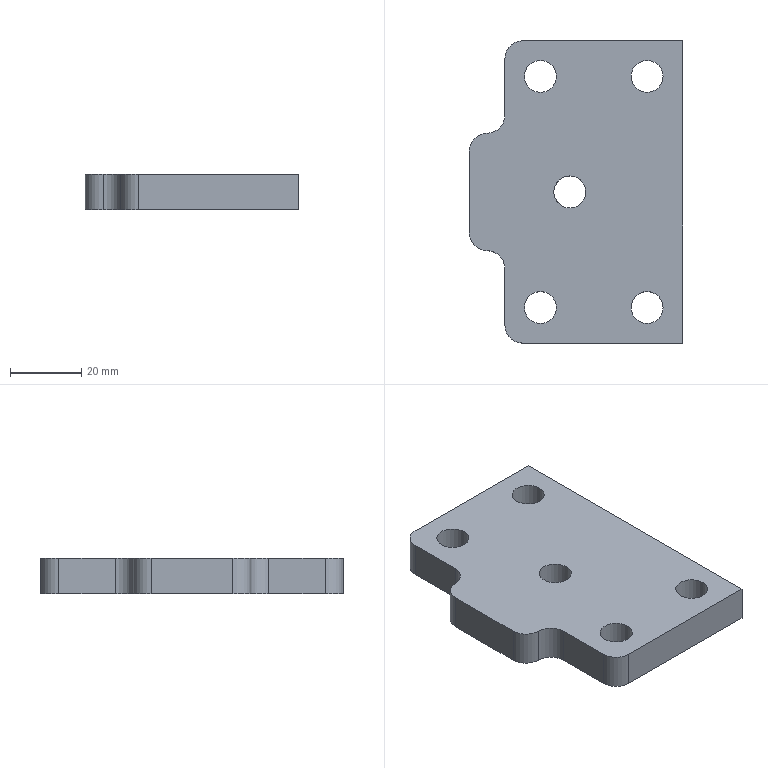Part | STEP file | PN_0048_id1026_x_t | 1 solid | 19 faces | box 60 x 85 x 10 mm | volume 42512 mm3 | cylinder 11 | plane 8 | commonest cylinder face diameters 10 x6 9 x5
STEP:
#1=CARTESIAN_POINT('',(294.75,11.5,105.));
#2=VERTEX_POINT('',#1);
#3=CARTESIAN_POINT('',(294.75,-11.5,105.));
#4=VERTEX_POINT('',#3);
#5=CARTESIAN_POINT('',(294.75,3.,105.));
#6=DIRECTION('',(0.,-1.,0.));
#7=VECTOR('',#6,1.);
#8=LINE('',#5,#7);
#9=EDGE_CURVE('',#2,#4,#8,.T.);
#10=ORIENTED_EDGE('',*,*,#9,.F.);
#11=CARTESIAN_POINT('',(294.75,11.5,95.));
#12=VERTEX_POINT('',#11);
#13=CARTESIAN_POINT('',(294.75,11.5,11.));
#14=DIRECTION('',(0.,0.,-1.));
#15=VECTOR('',#14,1.);
#16=LINE('',#13,#15);
#17=EDGE_CURVE('',#2,#12,#16,.T.);
#18=ORIENTED_EDGE('',*,*,#17,.T.);
#19=CARTESIAN_POINT('',(294.75,-11.5,95.));
#20=VERTEX_POINT('',#19);
#21=CARTESIAN_POINT('',(294.75,-13.,95.));
#22=DIRECTION('',(0.,-1.,0.));
#23=VECTOR('',#22,1.);
#24=LINE('',#21,#23);
#25=EDGE_CURVE('',#12,#20,#24,.T.);
#26=ORIENTED_EDGE('',*,*,#25,.T.);
#27=CARTESIAN_POINT('',(294.75,-11.5,105.));
#28=DIRECTION('',(0.,0.,1.));
#29=VECTOR('',#28,1.);
#30=LINE('',#27,#29);
#31=EDGE_CURVE('',#20,#4,#30,.T.);
#32=ORIENTED_EDGE('',*,*,#31,.T.);
#33=EDGE_LOOP('',(#10,#18,#26,#32));
#34=FACE_OUTER_BOUND('',#33,.T.);
#35=CARTESIAN_POINT('',(294.75,-13.,11.));
#36=DIRECTION('',(-1.,0.,0.));
#37=DIRECTION('',(0.,1.,0.));
#38=AXIS2_PLACEMENT_3D('',#35,#36,#37);
#39=PLANE('',#38);
#40=ADVANCED_FACE('',(#34),#39,.T.);
#41=CARTESIAN_POINT('',(354.75,-42.5,105.));
#42=VERTEX_POINT('',#41);
#43=CARTESIAN_POINT('',(309.75,-42.5,105.));
#44=VERTEX_POINT('',#43);
#45=CARTESIAN_POINT('',(546.19,-42.5,105.));
#46=DIRECTION('',(-1.,0.,0.));
#47=VECTOR('',#46,1.);
#48=LINE('',#45,#47);
#49=EDGE_CURVE('',#42,#44,#48,.T.);
#50=ORIENTED_EDGE('',*,*,#49,.T.);
#51=CARTESIAN_POINT('',(309.75,-42.5,95.));
#52=VERTEX_POINT('',#51);
#53=CARTESIAN_POINT('',(309.75,-42.5,95.));
#54=DIRECTION('',(0.,0.,-1.));
#55=VECTOR('',#54,1.);
#56=LINE('',#53,#55);
#57=EDGE_CURVE('',#44,#52,#56,.T.);
#58=ORIENTED_EDGE('',*,*,#57,.T.);
#59=CARTESIAN_POINT('',(354.75,-42.5,95.));
#60=VERTEX_POINT('',#59);
#61=CARTESIAN_POINT('',(265.5,-42.5,95.));
#62=DIRECTION('',(-1.,0.,0.));
#63=VECTOR('',#62,1.);
#64=LINE('',#61,#63);
#65=EDGE_CURVE('',#60,#52,#64,.T.);
#66=ORIENTED_EDGE('',*,*,#65,.F.);
#67=CARTESIAN_POINT('',(354.75,-42.5,11.));
#68=DIRECTION('',(0.,0.,1.));
#69=VECTOR('',#68,1.);
#70=LINE('',#67,#69);
#71=EDGE_CURVE('',#60,#42,#70,.T.);
#72=ORIENTED_EDGE('',*,*,#71,.T.);
#73=EDGE_LOOP('',(#50,#58,#66,#72));
#74=FACE_OUTER_BOUND('',#73,.T.);
#75=CARTESIAN_POINT('',(546.19,-42.5,11.));
#76=DIRECTION('',(0.,-1.,0.));
#77=DIRECTION('',(-1.,0.,0.));
#78=AXIS2_PLACEMENT_3D('',#75,#76,#77);
#79=PLANE('',#78);
#80=ADVANCED_FACE('',(#74),#79,.T.);
#81=CARTESIAN_POINT('',(354.75,42.5,95.));
#82=VERTEX_POINT('',#81);
#83=CARTESIAN_POINT('',(309.75,42.5,95.));
#84=VERTEX_POINT('',#83);
#85=CARTESIAN_POINT('',(265.5,42.5,95.));
#86=DIRECTION('',(-1.,0.,0.));
#87=VECTOR('',#86,1.);
#88=LINE('',#85,#87);
#89=EDGE_CURVE('',#82,#84,#88,.T.);
#90=ORIENTED_EDGE('',*,*,#89,.T.);
#91=CARTESIAN_POINT('',(309.75,42.5,105.));
#92=VERTEX_POINT('',#91);
#93=CARTESIAN_POINT('',(309.75,42.5,105.));
#94=DIRECTION('',(0.,0.,1.));
#95=VECTOR('',#94,1.);
#96=LINE('',#93,#95);
#97=EDGE_CURVE('',#84,#92,#96,.T.);
#98=ORIENTED_EDGE('',*,*,#97,.T.);
#99=CARTESIAN_POINT('',(354.75,42.5,105.));
#100=VERTEX_POINT('',#99);
#101=CARTESIAN_POINT('',(266.,42.5,105.));
#102=DIRECTION('',(-1.,0.,0.));
#103=VECTOR('',#102,1.);
#104=LINE('',#101,#103);
#105=EDGE_CURVE('',#100,#92,#104,.T.);
#106=ORIENTED_EDGE('',*,*,#105,.F.);
#107=CARTESIAN_POINT('',(354.75,42.5,11.));
#108=DIRECTION('',(0.,0.,1.));
#109=VECTOR('',#108,1.);
#110=LINE('',#107,#109);
#111=EDGE_CURVE('',#82,#100,#110,.T.);
#112=ORIENTED_EDGE('',*,*,#111,.F.);
#113=EDGE_LOOP('',(#90,#98,#106,#112));
#114=FACE_OUTER_BOUND('',#113,.T.);
#115=CARTESIAN_POINT('',(266.,42.5,11.));
#116=DIRECTION('',(0.,1.,0.));
#117=DIRECTION('',(1.,0.,0.));
#118=AXIS2_PLACEMENT_3D('',#115,#116,#117);
#119=PLANE('',#118);
#120=ADVANCED_FACE('',(#114),#119,.T.);
#121=CARTESIAN_POINT('',(323.,4.5,105.));
#122=VERTEX_POINT('',#121);
#123=CARTESIAN_POINT('',(323.,0.,105.));
#124=DIRECTION('',(0.,0.,-1.));
#125=DIRECTION('',(0.,1.,0.));
#126=AXIS2_PLACEMENT_3D('',#123,#124,#125);
#127=CIRCLE('',#126,4.5);
#128=EDGE_CURVE('',#122,#122,#127,.T.);
#129=ORIENTED_EDGE('',*,*,#128,.T.);
#130=EDGE_LOOP('',(#129));
#131=FACE_BOUND('',#130,.T.);
#132=CARTESIAN_POINT('',(319.25,-32.5,105.));
#133=VERTEX_POINT('',#132);
#134=CARTESIAN_POINT('',(314.75,-32.5,105.));
#135=DIRECTION('',(0.,0.,-1.));
#136=DIRECTION('',(1.,0.,0.));
#137=AXIS2_PLACEMENT_3D('',#134,#135,#136);
#138=CIRCLE('',#137,4.5);
#139=EDGE_CURVE('',#133,#133,#138,.T.);
#140=ORIENTED_EDGE('',*,*,#139,.T.);
#141=EDGE_LOOP('',(#140));
#142=FACE_BOUND('',#141,.T.);
#143=CARTESIAN_POINT('',(340.25,-32.5,105.));
#144=VERTEX_POINT('',#143);
#145=CARTESIAN_POINT('',(344.75,-32.5,105.));
#146=DIRECTION('',(0.,0.,1.));
#147=DIRECTION('',(-1.,0.,0.));
#148=AXIS2_PLACEMENT_3D('',#145,#146,#147);
#149=CIRCLE('',#148,4.5);
#150=EDGE_CURVE('',#144,#144,#149,.T.);
#151=ORIENTED_EDGE('',*,*,#150,.F.);
#152=EDGE_LOOP('',(#151));
#153=FACE_BOUND('',#152,.T.);
#154=CARTESIAN_POINT('',(319.25,32.5,105.));
#155=VERTEX_POINT('',#154);
#156=CARTESIAN_POINT('',(314.75,32.5,105.));
#157=DIRECTION('',(0.,0.,1.));
#158=DIRECTION('',(1.,0.,0.));
#159=AXIS2_PLACEMENT_3D('',#156,#157,#158);
#160=CIRCLE('',#159,4.5);
#161=EDGE_CURVE('',#155,#155,#160,.T.);
#162=ORIENTED_EDGE('',*,*,#161,.F.);
#163=EDGE_LOOP('',(#162));
#164=FACE_BOUND('',#163,.T.);
#165=CARTESIAN_POINT('',(340.25,32.5,105.));
#166=VERTEX_POINT('',#165);
#167=CARTESIAN_POINT('',(344.75,32.5,105.));
#168=DIRECTION('',(0.,0.,-1.));
#169=DIRECTION('',(-1.,0.,0.));
#170=AXIS2_PLACEMENT_3D('',#167,#168,#169);
#171=CIRCLE('',#170,4.5);
#172=EDGE_CURVE('',#166,#166,#171,.T.);
#173=ORIENTED_EDGE('',*,*,#172,.T.);
#174=EDGE_LOOP('',(#173));
#175=FACE_BOUND('',#174,.T.);
#176=ORIENTED_EDGE('',*,*,#105,.T.);
#177=CARTESIAN_POINT('',(304.75,37.5,105.));
#178=VERTEX_POINT('',#177);
#179=CARTESIAN_POINT('',(309.75,37.5,105.));
#180=DIRECTION('',(0.,0.,1.));
#181=DIRECTION('',(1.,0.,0.));
#182=AXIS2_PLACEMENT_3D('',#179,#180,#181);
#183=CIRCLE('',#182,5.);
#184=EDGE_CURVE('',#92,#178,#183,.T.);
#185=ORIENTED_EDGE('',*,*,#184,.T.);
#186=CARTESIAN_POINT('',(304.75,21.5,105.));
#187=VERTEX_POINT('',#186);
#188=CARTESIAN_POINT('',(304.75,3.,105.));
#189=DIRECTION('',(0.,-1.,0.));
#190=VECTOR('',#189,1.);
#191=LINE('',#188,#190);
#192=EDGE_CURVE('',#178,#187,#191,.T.);
#193=ORIENTED_EDGE('',*,*,#192,.T.);
#194=CARTESIAN_POINT('',(299.75,16.5,105.));
#195=VERTEX_POINT('',#194);
#196=CARTESIAN_POINT('',(299.75,21.5,105.));
#197=DIRECTION('',(0.,0.,-1.));
#198=DIRECTION('',(1.,0.,0.));
#199=AXIS2_PLACEMENT_3D('',#196,#197,#198);
#200=CIRCLE('',#199,5.);
#201=EDGE_CURVE('',#187,#195,#200,.T.);
#202=ORIENTED_EDGE('',*,*,#201,.T.);
#203=CARTESIAN_POINT('',(299.75,11.5,105.));
#204=DIRECTION('',(0.,0.,1.));
#205=DIRECTION('',(1.,0.,0.));
#206=AXIS2_PLACEMENT_3D('',#203,#204,#205);
#207=CIRCLE('',#206,5.);
#208=EDGE_CURVE('',#195,#2,#207,.T.);
#209=ORIENTED_EDGE('',*,*,#208,.T.);
#210=ORIENTED_EDGE('',*,*,#9,.T.);
#211=CARTESIAN_POINT('',(299.75,-16.5,105.));
#212=VERTEX_POINT('',#211);
#213=CARTESIAN_POINT('',(299.75,-11.5,105.));
#214=DIRECTION('',(0.,0.,1.));
#215=DIRECTION('',(1.,0.,0.));
#216=AXIS2_PLACEMENT_3D('',#213,#214,#215);
#217=CIRCLE('',#216,5.);
#218=EDGE_CURVE('',#4,#212,#217,.T.);
#219=ORIENTED_EDGE('',*,*,#218,.T.);
#220=CARTESIAN_POINT('',(304.75,-21.5,105.));
#221=VERTEX_POINT('',#220);
#222=CARTESIAN_POINT('',(299.75,-21.5,105.));
#223=DIRECTION('',(0.,0.,1.));
#224=DIRECTION('',(1.,0.,0.));
#225=AXIS2_PLACEMENT_3D('',#222,#223,#224);
#226=CIRCLE('',#225,5.);
#227=EDGE_CURVE('',#221,#212,#226,.T.);
#228=ORIENTED_EDGE('',*,*,#227,.F.);
#229=CARTESIAN_POINT('',(304.75,-37.5,105.));
#230=VERTEX_POINT('',#229);
#231=CARTESIAN_POINT('',(304.75,3.,105.));
#232=DIRECTION('',(0.,1.,0.));
#233=VECTOR('',#232,1.);
#234=LINE('',#231,#233);
#235=EDGE_CURVE('',#230,#221,#234,.T.);
#236=ORIENTED_EDGE('',*,*,#235,.F.);
#237=CARTESIAN_POINT('',(309.75,-37.5,105.));
#238=DIRECTION('',(0.,0.,1.));
#239=DIRECTION('',(1.,0.,0.));
#240=AXIS2_PLACEMENT_3D('',#237,#238,#239);
#241=CIRCLE('',#240,5.);
#242=EDGE_CURVE('',#230,#44,#241,.T.);
#243=ORIENTED_EDGE('',*,*,#242,.T.);
#244=ORIENTED_EDGE('',*,*,#49,.F.);
#245=CARTESIAN_POINT('',(354.75,52.192,105.));
#246=DIRECTION('',(0.,-1.,0.));
#247=VECTOR('',#246,1.);
#248=LINE('',#245,#247);
#249=EDGE_CURVE('',#100,#42,#248,.T.);
#250=ORIENTED_EDGE('',*,*,#249,.F.);
#251=EDGE_LOOP('',(#176,#185,#193,#202,#209,#210,#219,#228,#236,#243,#244,#250));
#252=FACE_BOUND('',#251,.T.);
#253=CARTESIAN_POINT('',(-321.,3.,105.));
#254=DIRECTION('',(0.,0.,1.));
#255=DIRECTION('',(1.,0.,0.));
#256=AXIS2_PLACEMENT_3D('',#253,#254,#255);
#257=PLANE('',#256);
#258=ADVANCED_FACE('',(#131,#142,#153,#164,#175,#252),#257,.T.);
#259=CARTESIAN_POINT('',(318.5,0.,95.));
#260=VERTEX_POINT('',#259);
#261=CARTESIAN_POINT('',(323.,0.,95.));
#262=DIRECTION('',(0.,0.,-1.));
#263=DIRECTION('',(-1.,0.,0.));
#264=AXIS2_PLACEMENT_3D('',#261,#262,#263);
#265=CIRCLE('',#264,4.5);
#266=EDGE_CURVE('',#260,#260,#265,.T.);
#267=ORIENTED_EDGE('',*,*,#266,.F.);
#268=EDGE_LOOP('',(#267));
#269=FACE_BOUND('',#268,.T.);
#270=CARTESIAN_POINT('',(310.25,-32.5,95.));
#271=VERTEX_POINT('',#270);
#272=CARTESIAN_POINT('',(314.75,-32.5,95.));
#273=DIRECTION('',(0.,0.,-1.));
#274=DIRECTION('',(-1.,0.,0.));
#275=AXIS2_PLACEMENT_3D('',#272,#273,#274);
#276=CIRCLE('',#275,4.5);
#277=EDGE_CURVE('',#271,#271,#276,.T.);
#278=ORIENTED_EDGE('',*,*,#277,.F.);
#279=EDGE_LOOP('',(#278));
#280=FACE_BOUND('',#279,.T.);
#281=CARTESIAN_POINT('',(340.25,-32.5,95.));
#282=VERTEX_POINT('',#281);
#283=CARTESIAN_POINT('',(344.75,-32.5,95.));
#284=DIRECTION('',(0.,0.,-1.));
#285=DIRECTION('',(-1.,0.,0.));
#286=AXIS2_PLACEMENT_3D('',#283,#284,#285);
#287=CIRCLE('',#286,4.5);
#288=EDGE_CURVE('',#282,#282,#287,.T.);
#289=ORIENTED_EDGE('',*,*,#288,.F.);
#290=EDGE_LOOP('',(#289));
#291=FACE_BOUND('',#290,.T.);
#292=CARTESIAN_POINT('',(310.25,32.5,95.));
#293=VERTEX_POINT('',#292);
#294=CARTESIAN_POINT('',(314.75,32.5,95.));
#295=DIRECTION('',(0.,0.,-1.));
#296=DIRECTION('',(-1.,0.,0.));
#297=AXIS2_PLACEMENT_3D('',#294,#295,#296);
#298=CIRCLE('',#297,4.5);
#299=EDGE_CURVE('',#293,#293,#298,.T.);
#300=ORIENTED_EDGE('',*,*,#299,.F.);
#301=EDGE_LOOP('',(#300));
#302=FACE_BOUND('',#301,.T.);
#303=CARTESIAN_POINT('',(340.25,32.5,95.));
#304=VERTEX_POINT('',#303);
#305=CARTESIAN_POINT('',(344.75,32.5,95.));
#306=DIRECTION('',(0.,0.,-1.));
#307=DIRECTION('',(-1.,0.,0.));
#308=AXIS2_PLACEMENT_3D('',#305,#306,#307);
#309=CIRCLE('',#308,4.5);
#310=EDGE_CURVE('',#304,#304,#309,.T.);
#311=ORIENTED_EDGE('',*,*,#310,.F.);
#312=EDGE_LOOP('',(#311));
#313=FACE_BOUND('',#312,.T.);
#314=CARTESIAN_POINT('',(304.75,21.5,95.));
#315=VERTEX_POINT('',#314);
#316=CARTESIAN_POINT('',(304.75,37.5,95.));
#317=VERTEX_POINT('',#316);
#318=CARTESIAN_POINT('',(304.75,3.,95.));
#319=DIRECTION('',(0.,1.,0.));
#320=VECTOR('',#319,1.);
#321=LINE('',#318,#320);
#322=EDGE_CURVE('',#315,#317,#321,.T.);
#323=ORIENTED_EDGE('',*,*,#322,.T.);
#324=CARTESIAN_POINT('',(309.75,37.5,95.));
#325=DIRECTION('',(0.,0.,-1.));
#326=DIRECTION('',(-1.,0.,0.));
#327=AXIS2_PLACEMENT_3D('',#324,#325,#326);
#328=CIRCLE('',#327,5.);
#329=EDGE_CURVE('',#317,#84,#328,.T.);
#330=ORIENTED_EDGE('',*,*,#329,.T.);
#331=ORIENTED_EDGE('',*,*,#89,.F.);
#332=CARTESIAN_POINT('',(354.75,3.,95.));
#333=DIRECTION('',(0.,-1.,0.));
#334=VECTOR('',#333,1.);
#335=LINE('',#332,#334);
#336=EDGE_CURVE('',#82,#60,#335,.T.);
#337=ORIENTED_EDGE('',*,*,#336,.T.);
#338=ORIENTED_EDGE('',*,*,#65,.T.);
#339=CARTESIAN_POINT('',(304.75,-37.5,95.));
#340=VERTEX_POINT('',#339);
#341=CARTESIAN_POINT('',(309.75,-37.5,95.));
#342=DIRECTION('',(0.,0.,-1.));
#343=DIRECTION('',(-1.,0.,0.));
#344=AXIS2_PLACEMENT_3D('',#341,#342,#343);
#345=CIRCLE('',#344,5.);
#346=EDGE_CURVE('',#52,#340,#345,.T.);
#347=ORIENTED_EDGE('',*,*,#346,.T.);
#348=CARTESIAN_POINT('',(304.75,-21.5,95.));
#349=VERTEX_POINT('',#348);
#350=CARTESIAN_POINT('',(304.75,3.,95.));
#351=DIRECTION('',(0.,-1.,0.));
#352=VECTOR('',#351,1.);
#353=LINE('',#350,#352);
#354=EDGE_CURVE('',#349,#340,#353,.T.);
#355=ORIENTED_EDGE('',*,*,#354,.F.);
#356=CARTESIAN_POINT('',(299.75,-16.5,95.));
#357=VERTEX_POINT('',#356);
#358=CARTESIAN_POINT('',(299.75,-21.5,95.));
#359=DIRECTION('',(0.,0.,-1.));
#360=DIRECTION('',(-1.,0.,0.));
#361=AXIS2_PLACEMENT_3D('',#358,#359,#360);
#362=CIRCLE('',#361,5.);
#363=EDGE_CURVE('',#357,#349,#362,.T.);
#364=ORIENTED_EDGE('',*,*,#363,.F.);
#365=CARTESIAN_POINT('',(299.75,-11.5,95.));
#366=DIRECTION('',(0.,0.,-1.));
#367=DIRECTION('',(-1.,0.,0.));
#368=AXIS2_PLACEMENT_3D('',#365,#366,#367);
#369=CIRCLE('',#368,5.);
#370=EDGE_CURVE('',#357,#20,#369,.T.);
#371=ORIENTED_EDGE('',*,*,#370,.T.);
#372=ORIENTED_EDGE('',*,*,#25,.F.);
#373=CARTESIAN_POINT('',(299.75,16.5,95.));
#374=VERTEX_POINT('',#373);
#375=CARTESIAN_POINT('',(299.75,11.5,95.));
#376=DIRECTION('',(0.,0.,-1.));
#377=DIRECTION('',(-1.,0.,0.));
#378=AXIS2_PLACEMENT_3D('',#375,#376,#377);
#379=CIRCLE('',#378,5.);
#380=EDGE_CURVE('',#12,#374,#379,.T.);
#381=ORIENTED_EDGE('',*,*,#380,.T.);
#382=CARTESIAN_POINT('',(299.75,21.5,95.));
#383=DIRECTION('',(0.,0.,1.));
#384=DIRECTION('',(-1.,0.,0.));
#385=AXIS2_PLACEMENT_3D('',#382,#383,#384);
#386=CIRCLE('',#385,5.);
#387=EDGE_CURVE('',#374,#315,#386,.T.);
#388=ORIENTED_EDGE('',*,*,#387,.T.);
#389=EDGE_LOOP('',(#323,#330,#331,#337,#338,#347,#355,#364,#371,#372,#381,#388));
#390=FACE_BOUND('',#389,.T.);
#391=CARTESIAN_POINT('',(265.5,3.,95.));
#392=DIRECTION('',(0.,0.,-1.));
#393=DIRECTION('',(-1.,0.,0.));
#394=AXIS2_PLACEMENT_3D('',#391,#392,#393);
#395=PLANE('',#394);
#396=ADVANCED_FACE('',(#269,#280,#291,#302,#313,#390),#395,.T.);
#397=ORIENTED_EDGE('',*,*,#111,.T.);
#398=ORIENTED_EDGE('',*,*,#249,.T.);
#399=ORIENTED_EDGE('',*,*,#71,.F.);
#400=ORIENTED_EDGE('',*,*,#336,.F.);
#401=EDGE_LOOP('',(#397,#398,#399,#400));
#402=FACE_OUTER_BOUND('',#401,.T.);
#403=CARTESIAN_POINT('',(354.75,52.192,11.));
#404=DIRECTION('',(-1.,0.,0.));
#405=DIRECTION('',(0.,1.,0.));
#406=AXIS2_PLACEMENT_3D('',#403,#404,#405);
#407=PLANE('',#406);
#408=ADVANCED_FACE('',(#402),#407,.F.);
#409=ORIENTED_EDGE('',*,*,#201,.F.);
#410=CARTESIAN_POINT('',(304.75,21.5,44.));
#411=DIRECTION('',(0.,0.,1.));
#412=VECTOR('',#411,1.);
#413=LINE('',#410,#412);
#414=EDGE_CURVE('',#315,#187,#413,.T.);
#415=ORIENTED_EDGE('',*,*,#414,.F.);
#416=ORIENTED_EDGE('',*,*,#387,.F.);
#417=CARTESIAN_POINT('',(299.75,16.5,44.));
#418=DIRECTION('',(0.,0.,1.));
#419=VECTOR('',#418,1.);
#420=LINE('',#417,#419);
#421=EDGE_CURVE('',#374,#195,#420,.T.);
#422=ORIENTED_EDGE('',*,*,#421,.T.);
#423=EDGE_LOOP('',(#409,#415,#416,#422));
#424=FACE_OUTER_BOUND('',#423,.T.);
#425=CARTESIAN_POINT('',(299.75,21.5,44.));
#426=DIRECTION('',(0.,0.,1.));
#427=DIRECTION('',(1.,0.,0.));
#428=AXIS2_PLACEMENT_3D('',#425,#426,#427);
#429=CYLINDRICAL_SURFACE('',#428,5.);
#430=ADVANCED_FACE('',(#424),#429,.F.);
#431=ORIENTED_EDGE('',*,*,#192,.F.);
#432=CARTESIAN_POINT('',(304.75,37.5,44.));
#433=DIRECTION('',(0.,0.,-1.));
#434=VECTOR('',#433,1.);
#435=LINE('',#432,#434);
#436=EDGE_CURVE('',#178,#317,#435,.T.);
#437=ORIENTED_EDGE('',*,*,#436,.T.);
#438=ORIENTED_EDGE('',*,*,#322,.F.);
#439=ORIENTED_EDGE('',*,*,#414,.T.);
#440=EDGE_LOOP('',(#431,#437,#438,#439));
#441=FACE_OUTER_BOUND('',#440,.T.);
#442=CARTESIAN_POINT('',(304.75,52.5,44.));
#443=DIRECTION('',(-1.,0.,0.));
#444=DIRECTION('',(0.,0.,1.));
#445=AXIS2_PLACEMENT_3D('',#442,#443,#444);
#446=PLANE('',#445);
#447=ADVANCED_FACE('',(#441),#446,.T.);
#448=ORIENTED_EDGE('',*,*,#227,.T.);
#449=CARTESIAN_POINT('',(299.75,-16.5,118.));
#450=DIRECTION('',(0.,0.,1.));
#451=VECTOR('',#450,1.);
#452=LINE('',#449,#451);
#453=EDGE_CURVE('',#357,#212,#452,.T.);
#454=ORIENTED_EDGE('',*,*,#453,.F.);
#455=ORIENTED_EDGE('',*,*,#363,.T.);
#456=CARTESIAN_POINT('',(304.75,-21.5,118.));
#457=DIRECTION('',(0.,0.,1.));
#458=VECTOR('',#457,1.);
#459=LINE('',#456,#458);
#460=EDGE_CURVE('',#349,#221,#459,.T.);
#461=ORIENTED_EDGE('',*,*,#460,.T.);
#462=EDGE_LOOP('',(#448,#454,#455,#461));
#463=FACE_OUTER_BOUND('',#462,.T.);
#464=CARTESIAN_POINT('',(299.75,-21.5,118.));
#465=DIRECTION('',(0.,0.,-1.));
#466=DIRECTION('',(-1.,0.,0.));
#467=AXIS2_PLACEMENT_3D('',#464,#465,#466);
#468=CYLINDRICAL_SURFACE('',#467,5.);
#469=ADVANCED_FACE('',(#463),#468,.F.);
#470=ORIENTED_EDGE('',*,*,#354,.T.);
#471=CARTESIAN_POINT('',(304.75,-37.5,11.));
#472=DIRECTION('',(0.,0.,1.));
#473=VECTOR('',#472,1.);
#474=LINE('',#471,#473);
#475=EDGE_CURVE('',#340,#230,#474,.T.);
#476=ORIENTED_EDGE('',*,*,#475,.T.);
#477=ORIENTED_EDGE('',*,*,#235,.T.);
#478=ORIENTED_EDGE('',*,*,#460,.F.);
#479=EDGE_LOOP('',(#470,#476,#477,#478));
#480=FACE_OUTER_BOUND('',#479,.T.);
#481=CARTESIAN_POINT('',(304.75,-52.5,118.));
#482=DIRECTION('',(1.,0.,0.));
#483=DIRECTION('',(0.,0.,-1.));
#484=AXIS2_PLACEMENT_3D('',#481,#482,#483);
#485=PLANE('',#484);
#486=ADVANCED_FACE('',(#480),#485,.F.);
#487=ORIENTED_EDGE('',*,*,#184,.F.);
#488=ORIENTED_EDGE('',*,*,#97,.F.);
#489=ORIENTED_EDGE('',*,*,#329,.F.);
#490=ORIENTED_EDGE('',*,*,#436,.F.);
#491=EDGE_LOOP('',(#487,#488,#489,#490));
#492=FACE_OUTER_BOUND('',#491,.T.);
#493=CARTESIAN_POINT('',(309.75,37.5,44.));
#494=DIRECTION('',(0.,0.,-1.));
#495=DIRECTION('',(-1.,0.,0.));
#496=AXIS2_PLACEMENT_3D('',#493,#494,#495);
#497=CYLINDRICAL_SURFACE('',#496,5.);
#498=ADVANCED_FACE('',(#492),#497,.T.);
#499=ORIENTED_EDGE('',*,*,#380,.F.);
#500=ORIENTED_EDGE('',*,*,#17,.F.);
#501=ORIENTED_EDGE('',*,*,#208,.F.);
#502=ORIENTED_EDGE('',*,*,#421,.F.);
#503=EDGE_LOOP('',(#499,#500,#501,#502));
#504=FACE_OUTER_BOUND('',#503,.T.);
#505=CARTESIAN_POINT('',(299.75,11.5,44.));
#506=DIRECTION('',(0.,0.,1.));
#507=DIRECTION('',(1.,0.,0.));
#508=AXIS2_PLACEMENT_3D('',#505,#506,#507);
#509=CYLINDRICAL_SURFACE('',#508,5.);
#510=ADVANCED_FACE('',(#504),#509,.T.);
#511=ORIENTED_EDGE('',*,*,#242,.F.);
#512=ORIENTED_EDGE('',*,*,#475,.F.);
#513=ORIENTED_EDGE('',*,*,#346,.F.);
#514=ORIENTED_EDGE('',*,*,#57,.F.);
#515=EDGE_LOOP('',(#511,#512,#513,#514));
#516=FACE_OUTER_BOUND('',#515,.T.);
#517=CARTESIAN_POINT('',(309.75,-37.5,11.));
#518=DIRECTION('',(0.,0.,1.));
#519=DIRECTION('',(1.,0.,0.));
#520=AXIS2_PLACEMENT_3D('',#517,#518,#519);
#521=CYLINDRICAL_SURFACE('',#520,5.);
#522=ADVANCED_FACE('',(#516),#521,.T.);
#523=ORIENTED_EDGE('',*,*,#370,.F.);
#524=ORIENTED_EDGE('',*,*,#453,.T.);
#525=ORIENTED_EDGE('',*,*,#218,.F.);
#526=ORIENTED_EDGE('',*,*,#31,.F.);
#527=EDGE_LOOP('',(#523,#524,#525,#526));
#528=FACE_OUTER_BOUND('',#527,.T.);
#529=CARTESIAN_POINT('',(299.75,-11.5,11.));
#530=DIRECTION('',(0.,0.,-1.));
#531=DIRECTION('',(-1.,0.,0.));
#532=AXIS2_PLACEMENT_3D('',#529,#530,#531);
#533=CYLINDRICAL_SURFACE('',#532,5.);
#534=ADVANCED_FACE('',(#528),#533,.T.);
#535=ORIENTED_EDGE('',*,*,#310,.T.);
#536=EDGE_LOOP('',(#535));
#537=FACE_BOUND('',#536,.T.);
#538=ORIENTED_EDGE('',*,*,#172,.F.);
#539=EDGE_LOOP('',(#538));
#540=FACE_BOUND('',#539,.T.);
#541=CARTESIAN_POINT('',(344.75,32.5,105.));
#542=DIRECTION('',(0.,0.,-1.));
#543=DIRECTION('',(-1.,0.,0.));
#544=AXIS2_PLACEMENT_3D('',#541,#542,#543);
#545=CYLINDRICAL_SURFACE('',#544,4.5);
#546=ADVANCED_FACE('',(#537,#540),#545,.F.);
#547=ORIENTED_EDGE('',*,*,#299,.T.);
#548=EDGE_LOOP('',(#547));
#549=FACE_BOUND('',#548,.T.);
#550=ORIENTED_EDGE('',*,*,#161,.T.);
#551=EDGE_LOOP('',(#550));
#552=FACE_BOUND('',#551,.T.);
#553=CARTESIAN_POINT('',(314.75,32.5,105.));
#554=DIRECTION('',(0.,0.,-1.));
#555=DIRECTION('',(1.,0.,0.));
#556=AXIS2_PLACEMENT_3D('',#553,#554,#555);
#557=CYLINDRICAL_SURFACE('',#556,4.5);
#558=ADVANCED_FACE('',(#549,#552),#557,.F.);
#559=ORIENTED_EDGE('',*,*,#288,.T.);
#560=EDGE_LOOP('',(#559));
#561=FACE_BOUND('',#560,.T.);
#562=ORIENTED_EDGE('',*,*,#150,.T.);
#563=EDGE_LOOP('',(#562));
#564=FACE_BOUND('',#563,.T.);
#565=CARTESIAN_POINT('',(344.75,-32.5,105.));
#566=DIRECTION('',(0.,0.,-1.));
#567=DIRECTION('',(-1.,0.,0.));
#568=AXIS2_PLACEMENT_3D('',#565,#566,#567);
#569=CYLINDRICAL_SURFACE('',#568,4.5);
#570=ADVANCED_FACE('',(#561,#564),#569,.F.);
#571=ORIENTED_EDGE('',*,*,#277,.T.);
#572=EDGE_LOOP('',(#571));
#573=FACE_BOUND('',#572,.T.);
#574=ORIENTED_EDGE('',*,*,#139,.F.);
#575=EDGE_LOOP('',(#574));
#576=FACE_BOUND('',#575,.T.);
#577=CARTESIAN_POINT('',(314.75,-32.5,105.));
#578=DIRECTION('',(0.,0.,-1.));
#579=DIRECTION('',(1.,0.,0.));
#580=AXIS2_PLACEMENT_3D('',#577,#578,#579);
#581=CYLINDRICAL_SURFACE('',#580,4.5);
#582=ADVANCED_FACE('',(#573,#576),#581,.F.);
#583=ORIENTED_EDGE('',*,*,#266,.T.);
#584=EDGE_LOOP('',(#583));
#585=FACE_BOUND('',#584,.T.);
#586=ORIENTED_EDGE('',*,*,#128,.F.);
#587=EDGE_LOOP('',(#586));
#588=FACE_BOUND('',#587,.T.);
#589=CARTESIAN_POINT('',(323.,0.,105.));
#590=DIRECTION('',(0.,0.,-1.));
#591=DIRECTION('',(0.,1.,0.));
#592=AXIS2_PLACEMENT_3D('',#589,#590,#591);
#593=CYLINDRICAL_SURFACE('',#592,4.5);
#594=ADVANCED_FACE('',(#585,#588),#593,.F.);
#595=CLOSED_SHELL('',(#40,#80,#120,#258,#396,#408,#430,#447,#469,#486,#498,#510,#522,#534,#546,#558,#570,#582,#594));
#596=MANIFOLD_SOLID_BREP('',#595);
#597=(LENGTH_UNIT()NAMED_UNIT(*)SI_UNIT(.MILLI.,.METRE.));
#598=UNCERTAINTY_MEASURE_WITH_UNIT(LENGTH_MEASURE(0.00002),#597,'','');
#599=(NAMED_UNIT(*)PLANE_ANGLE_UNIT()SI_UNIT($,.RADIAN.));
#600=PLANE_ANGLE_MEASURE_WITH_UNIT(PLANE_ANGLE_MEASURE(0.01745),#599);
#601=DIMENSIONAL_EXPONENTS(0.,0.,0.,0.,0.,0.,0.);
#602=(CONVERSION_BASED_UNIT('DEGREE',#600)NAMED_UNIT(#601)PLANE_ANGLE_UNIT());
#603=(NAMED_UNIT(*)SI_UNIT($,.STERADIAN.)SOLID_ANGLE_UNIT());
#604=(GEOMETRIC_REPRESENTATION_CONTEXT(3)GLOBAL_UNCERTAINTY_ASSIGNED_CONTEXT((#598))GLOBAL_UNIT_ASSIGNED_CONTEXT((#597,#602,#603))REPRESENTATION_CONTEXT('',''));
#605=ADVANCED_BREP_SHAPE_REPRESENTATION('',(#596),#604);